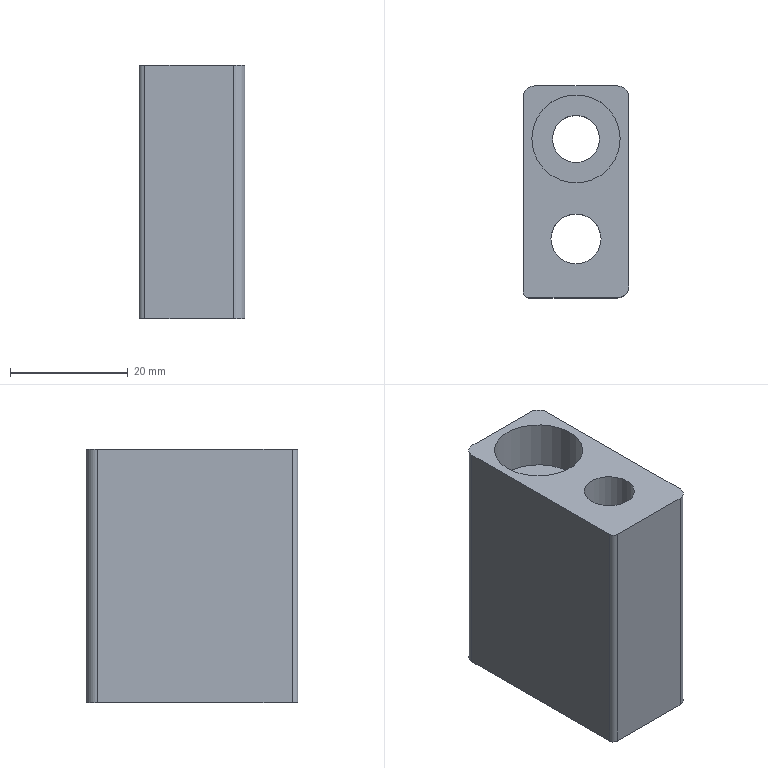Part | NX | features PH-18 2 | 1 solid | 16 faces | box 18 x 36 x 43 mm | volume 20467 mm3 | cylinder 8 | plane 8 | commonest cylinder face diameters 4 x3 2 x1 8.001 x1 8.5 x1 14.5 x1 15 x1
STEP:
#1=CARTESIAN_POINT('',(4143.236,-904.122,902.716));
#2=VERTEX_POINT('',#1);
#3=CARTESIAN_POINT('',(4145.236,-902.122,902.716));
#4=VERTEX_POINT('',#3);
#5=CARTESIAN_POINT('',(4143.236,-902.122,902.716));
#6=DIRECTION('',(0.,0.,-1.));
#7=DIRECTION('',(-1.,0.,0.));
#8=AXIS2_PLACEMENT_3D('',#5,#6,#7);
#9=CIRCLE('',#8,2.);
#10=EDGE_CURVE('',#2,#4,#9,.F.);
#11=ORIENTED_EDGE('',*,*,#10,.T.);
#12=CARTESIAN_POINT('',(4145.236,-902.122,945.716));
#13=VERTEX_POINT('',#12);
#14=CARTESIAN_POINT('',(4145.236,-902.122,915.716));
#15=DIRECTION('',(0.,0.,1.));
#16=VECTOR('',#15,1000.);
#17=LINE('',#14,#16);
#18=EDGE_CURVE('',#4,#13,#17,.T.);
#19=ORIENTED_EDGE('',*,*,#18,.T.);
#20=CARTESIAN_POINT('',(4143.236,-904.122,945.716));
#21=VERTEX_POINT('',#20);
#22=CARTESIAN_POINT('',(4143.236,-902.122,945.716));
#23=DIRECTION('',(0.,0.,-1.));
#24=DIRECTION('',(1.,0.,0.));
#25=AXIS2_PLACEMENT_3D('',#22,#23,#24);
#26=CIRCLE('',#25,2.);
#27=EDGE_CURVE('',#13,#21,#26,.T.);
#28=ORIENTED_EDGE('',*,*,#27,.T.);
#29=CARTESIAN_POINT('',(4143.236,-904.122,915.716));
#30=DIRECTION('',(0.,0.,1.));
#31=VECTOR('',#30,1000.);
#32=LINE('',#29,#31);
#33=EDGE_CURVE('',#21,#2,#32,.F.);
#34=ORIENTED_EDGE('',*,*,#33,.T.);
#35=EDGE_LOOP('',(#11,#19,#28,#34));
#36=FACE_BOUND('',#35,.T.);
#37=CARTESIAN_POINT('',(4143.236,-902.122,915.716));
#38=DIRECTION('',(0.,0.,1.));
#39=DIRECTION('',(1.,0.,0.));
#40=AXIS2_PLACEMENT_3D('',#37,#38,#39);
#41=CYLINDRICAL_SURFACE('',#40,2.);
#42=ADVANCED_FACE('',(#36),#41,.T.);
#43=CARTESIAN_POINT('',(4143.236,-868.122,902.716));
#44=VERTEX_POINT('',#43);
#45=CARTESIAN_POINT('',(4129.236,-868.122,902.716));
#46=VERTEX_POINT('',#45);
#47=CARTESIAN_POINT('',(4136.236,-868.122,902.716));
#48=DIRECTION('',(1.,0.,0.));
#49=VECTOR('',#48,1000.);
#50=LINE('',#47,#49);
#51=EDGE_CURVE('',#44,#46,#50,.F.);
#52=ORIENTED_EDGE('',*,*,#51,.T.);
#53=CARTESIAN_POINT('',(4129.236,-868.122,945.716));
#54=VERTEX_POINT('',#53);
#55=CARTESIAN_POINT('',(4129.236,-868.122,915.716));
#56=DIRECTION('',(0.,0.,1.));
#57=VECTOR('',#56,1000.);
#58=LINE('',#55,#57);
#59=EDGE_CURVE('',#54,#46,#58,.F.);
#60=ORIENTED_EDGE('',*,*,#59,.F.);
#61=CARTESIAN_POINT('',(4143.236,-868.122,945.716));
#62=VERTEX_POINT('',#61);
#63=CARTESIAN_POINT('',(4136.236,-868.122,945.716));
#64=DIRECTION('',(-1.,0.,0.));
#65=VECTOR('',#64,1000.);
#66=LINE('',#63,#65);
#67=EDGE_CURVE('',#54,#62,#66,.F.);
#68=ORIENTED_EDGE('',*,*,#67,.T.);
#69=CARTESIAN_POINT('',(4143.236,-868.122,915.716));
#70=DIRECTION('',(0.,0.,1.));
#71=VECTOR('',#70,1000.);
#72=LINE('',#69,#71);
#73=EDGE_CURVE('',#44,#62,#72,.T.);
#74=ORIENTED_EDGE('',*,*,#73,.F.);
#75=EDGE_LOOP('',(#52,#60,#68,#74));
#76=FACE_BOUND('',#75,.T.);
#77=CARTESIAN_POINT('',(4136.236,-868.122,915.716));
#78=DIRECTION('',(0.,1.,0.));
#79=DIRECTION('',(0.,0.,-1.));
#80=AXIS2_PLACEMENT_3D('',#77,#78,#79);
#81=PLANE('',#80);
#82=ADVANCED_FACE('',(#76),#81,.T.);
#83=CARTESIAN_POINT('',(4127.236,-870.122,902.716));
#84=VERTEX_POINT('',#83);
#85=CARTESIAN_POINT('',(4129.236,-870.122,902.716));
#86=DIRECTION('',(0.,0.,-1.));
#87=DIRECTION('',(-1.,0.,0.));
#88=AXIS2_PLACEMENT_3D('',#85,#86,#87);
#89=CIRCLE('',#88,2.);
#90=EDGE_CURVE('',#46,#84,#89,.F.);
#91=ORIENTED_EDGE('',*,*,#90,.T.);
#92=CARTESIAN_POINT('',(4127.236,-870.122,945.716));
#93=VERTEX_POINT('',#92);
#94=CARTESIAN_POINT('',(4127.236,-870.122,915.716));
#95=DIRECTION('',(0.,0.,1.));
#96=VECTOR('',#95,1000.);
#97=LINE('',#94,#96);
#98=EDGE_CURVE('',#84,#93,#97,.T.);
#99=ORIENTED_EDGE('',*,*,#98,.T.);
#100=CARTESIAN_POINT('',(4129.236,-870.122,945.716));
#101=DIRECTION('',(0.,0.,-1.));
#102=DIRECTION('',(1.,0.,0.));
#103=AXIS2_PLACEMENT_3D('',#100,#101,#102);
#104=CIRCLE('',#103,2.);
#105=EDGE_CURVE('',#93,#54,#104,.T.);
#106=ORIENTED_EDGE('',*,*,#105,.T.);
#107=ORIENTED_EDGE('',*,*,#59,.T.);
#108=EDGE_LOOP('',(#91,#99,#106,#107));
#109=FACE_BOUND('',#108,.T.);
#110=CARTESIAN_POINT('',(4129.236,-870.122,915.716));
#111=DIRECTION('',(0.,0.,1.));
#112=DIRECTION('',(1.,0.,0.));
#113=AXIS2_PLACEMENT_3D('',#110,#111,#112);
#114=CYLINDRICAL_SURFACE('',#113,2.);
#115=ADVANCED_FACE('',(#109),#114,.T.);
#116=CARTESIAN_POINT('',(4127.236,-903.122,945.716));
#117=VERTEX_POINT('',#116);
#118=CARTESIAN_POINT('',(4127.236,-885.622,945.716));
#119=DIRECTION('',(0.,-1.,0.));
#120=VECTOR('',#119,1000.);
#121=LINE('',#118,#120);
#122=EDGE_CURVE('',#117,#93,#121,.F.);
#123=ORIENTED_EDGE('',*,*,#122,.T.);
#124=ORIENTED_EDGE('',*,*,#98,.F.);
#125=CARTESIAN_POINT('',(4127.236,-903.122,902.716));
#126=VERTEX_POINT('',#125);
#127=CARTESIAN_POINT('',(4127.236,-885.622,902.716));
#128=DIRECTION('',(0.,1.,0.));
#129=VECTOR('',#128,1000.);
#130=LINE('',#127,#129);
#131=EDGE_CURVE('',#126,#84,#130,.T.);
#132=ORIENTED_EDGE('',*,*,#131,.F.);
#133=CARTESIAN_POINT('',(4127.236,-903.122,915.716));
#134=DIRECTION('',(0.,0.,1.));
#135=VECTOR('',#134,1000.);
#136=LINE('',#133,#135);
#137=EDGE_CURVE('',#117,#126,#136,.F.);
#138=ORIENTED_EDGE('',*,*,#137,.F.);
#139=EDGE_LOOP('',(#123,#124,#132,#138));
#140=FACE_BOUND('',#139,.T.);
#141=CARTESIAN_POINT('',(4127.236,-885.622,915.716));
#142=DIRECTION('',(-1.,0.,0.));
#143=DIRECTION('',(0.,0.,1.));
#144=AXIS2_PLACEMENT_3D('',#141,#142,#143);
#145=PLANE('',#144);
#146=ADVANCED_FACE('',(#140),#145,.T.);
#147=CARTESIAN_POINT('',(4145.236,-870.122,902.716));
#148=VERTEX_POINT('',#147);
#149=CARTESIAN_POINT('',(4143.236,-870.122,902.716));
#150=DIRECTION('',(0.,0.,-1.));
#151=DIRECTION('',(-1.,0.,0.));
#152=AXIS2_PLACEMENT_3D('',#149,#150,#151);
#153=CIRCLE('',#152,2.);
#154=EDGE_CURVE('',#148,#44,#153,.F.);
#155=ORIENTED_EDGE('',*,*,#154,.T.);
#156=ORIENTED_EDGE('',*,*,#73,.T.);
#157=CARTESIAN_POINT('',(4145.236,-870.122,945.716));
#158=VERTEX_POINT('',#157);
#159=CARTESIAN_POINT('',(4143.236,-870.122,945.716));
#160=DIRECTION('',(0.,0.,-1.));
#161=DIRECTION('',(1.,0.,0.));
#162=AXIS2_PLACEMENT_3D('',#159,#160,#161);
#163=CIRCLE('',#162,2.);
#164=EDGE_CURVE('',#158,#62,#163,.F.);
#165=ORIENTED_EDGE('',*,*,#164,.F.);
#166=CARTESIAN_POINT('',(4145.236,-870.122,915.716));
#167=DIRECTION('',(0.,0.,1.));
#168=VECTOR('',#167,1000.);
#169=LINE('',#166,#168);
#170=EDGE_CURVE('',#158,#148,#169,.F.);
#171=ORIENTED_EDGE('',*,*,#170,.T.);
#172=EDGE_LOOP('',(#155,#156,#165,#171));
#173=FACE_BOUND('',#172,.T.);
#174=CARTESIAN_POINT('',(4143.236,-870.122,915.716));
#175=DIRECTION('',(0.,0.,1.));
#176=DIRECTION('',(1.,0.,0.));
#177=AXIS2_PLACEMENT_3D('',#174,#175,#176);
#178=CYLINDRICAL_SURFACE('',#177,2.);
#179=ADVANCED_FACE('',(#173),#178,.T.);
#180=CARTESIAN_POINT('',(4128.236,-904.122,902.716));
#181=VERTEX_POINT('',#180);
#182=CARTESIAN_POINT('',(4136.236,-904.122,902.716));
#183=DIRECTION('',(-1.,0.,0.));
#184=VECTOR('',#183,1000.);
#185=LINE('',#182,#184);
#186=EDGE_CURVE('',#181,#2,#185,.F.);
#187=ORIENTED_EDGE('',*,*,#186,.T.);
#188=ORIENTED_EDGE('',*,*,#33,.F.);
#189=CARTESIAN_POINT('',(4128.236,-904.122,945.716));
#190=VERTEX_POINT('',#189);
#191=CARTESIAN_POINT('',(4136.236,-904.122,945.716));
#192=DIRECTION('',(1.,0.,0.));
#193=VECTOR('',#192,1000.);
#194=LINE('',#191,#193);
#195=EDGE_CURVE('',#21,#190,#194,.F.);
#196=ORIENTED_EDGE('',*,*,#195,.T.);
#197=CARTESIAN_POINT('',(4128.236,-904.122,915.716));
#198=DIRECTION('',(0.,0.,1.));
#199=VECTOR('',#198,1000.);
#200=LINE('',#197,#199);
#201=EDGE_CURVE('',#181,#190,#200,.T.);
#202=ORIENTED_EDGE('',*,*,#201,.F.);
#203=EDGE_LOOP('',(#187,#188,#196,#202));
#204=FACE_BOUND('',#203,.T.);
#205=CARTESIAN_POINT('',(4136.236,-904.122,915.716));
#206=DIRECTION('',(0.,-1.,0.));
#207=DIRECTION('',(0.,0.,1.));
#208=AXIS2_PLACEMENT_3D('',#205,#206,#207);
#209=PLANE('',#208);
#210=ADVANCED_FACE('',(#204),#209,.T.);
#211=CARTESIAN_POINT('',(4145.236,-885.622,902.716));
#212=DIRECTION('',(0.,-1.,0.));
#213=VECTOR('',#212,1000.);
#214=LINE('',#211,#213);
#215=EDGE_CURVE('',#4,#148,#214,.F.);
#216=ORIENTED_EDGE('',*,*,#215,.T.);
#217=ORIENTED_EDGE('',*,*,#170,.F.);
#218=CARTESIAN_POINT('',(4145.236,-885.622,945.716));
#219=DIRECTION('',(0.,1.,0.));
#220=VECTOR('',#219,1000.);
#221=LINE('',#218,#220);
#222=EDGE_CURVE('',#158,#13,#221,.F.);
#223=ORIENTED_EDGE('',*,*,#222,.T.);
#224=ORIENTED_EDGE('',*,*,#18,.F.);
#225=EDGE_LOOP('',(#216,#217,#223,#224));
#226=FACE_BOUND('',#225,.T.);
#227=CARTESIAN_POINT('',(4145.236,-885.622,915.716));
#228=DIRECTION('',(1.,0.,0.));
#229=DIRECTION('',(0.,0.,-1.));
#230=AXIS2_PLACEMENT_3D('',#227,#228,#229);
#231=PLANE('',#230);
#232=ADVANCED_FACE('',(#226),#231,.T.);
#233=CARTESIAN_POINT('',(4128.236,-903.122,902.716));
#234=DIRECTION('',(0.,0.,-1.));
#235=DIRECTION('',(-1.,0.,0.));
#236=AXIS2_PLACEMENT_3D('',#233,#234,#235);
#237=CIRCLE('',#236,1.);
#238=EDGE_CURVE('',#126,#181,#237,.F.);
#239=ORIENTED_EDGE('',*,*,#238,.T.);
#240=ORIENTED_EDGE('',*,*,#201,.T.);
#241=CARTESIAN_POINT('',(4128.236,-903.122,945.716));
#242=DIRECTION('',(0.,0.,-1.));
#243=DIRECTION('',(1.,0.,0.));
#244=AXIS2_PLACEMENT_3D('',#241,#242,#243);
#245=CIRCLE('',#244,1.);
#246=EDGE_CURVE('',#190,#117,#245,.T.);
#247=ORIENTED_EDGE('',*,*,#246,.T.);
#248=ORIENTED_EDGE('',*,*,#137,.T.);
#249=EDGE_LOOP('',(#239,#240,#247,#248));
#250=FACE_BOUND('',#249,.T.);
#251=CARTESIAN_POINT('',(4128.236,-903.122,915.716));
#252=DIRECTION('',(0.,0.,1.));
#253=DIRECTION('',(1.,0.,0.));
#254=AXIS2_PLACEMENT_3D('',#251,#252,#253);
#255=CYLINDRICAL_SURFACE('',#254,1.);
#256=ADVANCED_FACE('',(#250),#255,.T.);
#257=CARTESIAN_POINT('',(4132.236,-877.122,902.716));
#258=VERTEX_POINT('',#257);
#259=CARTESIAN_POINT('',(4136.236,-877.122,902.716));
#260=DIRECTION('',(0.,0.,-1.));
#261=DIRECTION('',(-1.,0.,0.));
#262=AXIS2_PLACEMENT_3D('',#259,#260,#261);
#263=CIRCLE('',#262,4.);
#264=EDGE_CURVE('',#258,#258,#263,.T.);
#265=ORIENTED_EDGE('',*,*,#264,.T.);
#266=EDGE_LOOP('',(#265));
#267=FACE_BOUND('',#266,.T.);
#268=CARTESIAN_POINT('',(4132.236,-877.122,937.416));
#269=VERTEX_POINT('',#268);
#270=CARTESIAN_POINT('',(4136.236,-877.122,937.416));
#271=DIRECTION('',(0.,0.,-1.));
#272=DIRECTION('',(-1.,0.,0.));
#273=AXIS2_PLACEMENT_3D('',#270,#271,#272);
#274=CIRCLE('',#273,4.);
#275=EDGE_CURVE('',#269,#269,#274,.T.);
#276=ORIENTED_EDGE('',*,*,#275,.F.);
#277=EDGE_LOOP('',(#276));
#278=FACE_BOUND('',#277,.T.);
#279=CARTESIAN_POINT('',(4136.236,-877.122,945.716));
#280=DIRECTION('',(0.,0.,-1.));
#281=DIRECTION('',(1.,0.,0.));
#282=AXIS2_PLACEMENT_3D('',#279,#280,#281);
#283=CYLINDRICAL_SURFACE('',#282,4.);
#284=ADVANCED_FACE('',(#267,#278),#283,.F.);
#285=CARTESIAN_POINT('',(4143.486,-894.122,902.716));
#286=VERTEX_POINT('',#285);
#287=CARTESIAN_POINT('',(4136.236,-894.122,902.716));
#288=DIRECTION('',(0.,0.,1.));
#289=DIRECTION('',(1.,0.,0.));
#290=AXIS2_PLACEMENT_3D('',#287,#288,#289);
#291=CIRCLE('',#290,7.25);
#292=EDGE_CURVE('',#286,#286,#291,.T.);
#293=ORIENTED_EDGE('',*,*,#292,.T.);
#294=EDGE_LOOP('',(#293));
#295=FACE_BOUND('',#294,.T.);
#296=ORIENTED_EDGE('',*,*,#154,.F.);
#297=ORIENTED_EDGE('',*,*,#215,.F.);
#298=ORIENTED_EDGE('',*,*,#10,.F.);
#299=ORIENTED_EDGE('',*,*,#186,.F.);
#300=ORIENTED_EDGE('',*,*,#238,.F.);
#301=ORIENTED_EDGE('',*,*,#131,.T.);
#302=ORIENTED_EDGE('',*,*,#90,.F.);
#303=ORIENTED_EDGE('',*,*,#51,.F.);
#304=EDGE_LOOP('',(#296,#297,#298,#299,#300,#301,#302,#303));
#305=FACE_BOUND('',#304,.T.);
#306=ORIENTED_EDGE('',*,*,#264,.F.);
#307=EDGE_LOOP('',(#306));
#308=FACE_BOUND('',#307,.T.);
#309=CARTESIAN_POINT('',(4123.486,-858.122,902.716));
#310=DIRECTION('',(0.,0.,-1.));
#311=DIRECTION('',(-1.,0.,0.));
#312=AXIS2_PLACEMENT_3D('',#309,#310,#311);
#313=PLANE('',#312);
#314=ADVANCED_FACE('',(#295,#305,#308),#313,.T.);
#315=ORIENTED_EDGE('',*,*,#275,.T.);
#316=EDGE_LOOP('',(#315));
#317=FACE_BOUND('',#316,.T.);
#318=CARTESIAN_POINT('',(4143.736,-877.122,937.416));
#319=VERTEX_POINT('',#318);
#320=CARTESIAN_POINT('',(4136.236,-877.122,937.416));
#321=DIRECTION('',(0.,0.,1.));
#322=DIRECTION('',(1.,0.,0.));
#323=AXIS2_PLACEMENT_3D('',#320,#321,#322);
#324=CIRCLE('',#323,7.5);
#325=EDGE_CURVE('',#319,#319,#324,.T.);
#326=ORIENTED_EDGE('',*,*,#325,.T.);
#327=EDGE_LOOP('',(#326));
#328=FACE_BOUND('',#327,.T.);
#329=CARTESIAN_POINT('',(4136.236,-877.122,937.416));
#330=DIRECTION('',(0.,0.,-1.));
#331=DIRECTION('',(-1.,0.,0.));
#332=AXIS2_PLACEMENT_3D('',#329,#330,#331);
#333=PLANE('',#332);
#334=ADVANCED_FACE('',(#317,#328),#333,.F.);
#335=CARTESIAN_POINT('',(4143.736,-877.122,945.716));
#336=VERTEX_POINT('',#335);
#337=CARTESIAN_POINT('',(4136.236,-877.122,945.716));
#338=DIRECTION('',(0.,0.,-1.));
#339=DIRECTION('',(1.,0.,0.));
#340=AXIS2_PLACEMENT_3D('',#337,#338,#339);
#341=CIRCLE('',#340,7.5);
#342=EDGE_CURVE('',#336,#336,#341,.T.);
#343=ORIENTED_EDGE('',*,*,#342,.F.);
#344=EDGE_LOOP('',(#343));
#345=FACE_BOUND('',#344,.T.);
#346=ORIENTED_EDGE('',*,*,#325,.F.);
#347=EDGE_LOOP('',(#346));
#348=FACE_BOUND('',#347,.T.);
#349=CARTESIAN_POINT('',(4136.236,-877.122,945.716));
#350=DIRECTION('',(0.,0.,-1.));
#351=DIRECTION('',(1.,0.,0.));
#352=AXIS2_PLACEMENT_3D('',#349,#350,#351);
#353=CYLINDRICAL_SURFACE('',#352,7.5);
#354=ADVANCED_FACE('',(#345,#348),#353,.F.);
#355=CARTESIAN_POINT('',(4140.486,-894.122,945.716));
#356=VERTEX_POINT('',#355);
#357=CARTESIAN_POINT('',(4136.236,-894.122,945.716));
#358=DIRECTION('',(0.,0.,1.));
#359=DIRECTION('',(1.,0.,0.));
#360=AXIS2_PLACEMENT_3D('',#357,#358,#359);
#361=CIRCLE('',#360,4.25);
#362=EDGE_CURVE('',#356,#356,#361,.T.);
#363=ORIENTED_EDGE('',*,*,#362,.F.);
#364=EDGE_LOOP('',(#363));
#365=FACE_BOUND('',#364,.T.);
#366=ORIENTED_EDGE('',*,*,#164,.T.);
#367=ORIENTED_EDGE('',*,*,#67,.F.);
#368=ORIENTED_EDGE('',*,*,#105,.F.);
#369=ORIENTED_EDGE('',*,*,#122,.F.);
#370=ORIENTED_EDGE('',*,*,#246,.F.);
#371=ORIENTED_EDGE('',*,*,#195,.F.);
#372=ORIENTED_EDGE('',*,*,#27,.F.);
#373=ORIENTED_EDGE('',*,*,#222,.F.);
#374=EDGE_LOOP('',(#366,#367,#368,#369,#370,#371,#372,#373));
#375=FACE_BOUND('',#374,.T.);
#376=ORIENTED_EDGE('',*,*,#342,.T.);
#377=EDGE_LOOP('',(#376));
#378=FACE_BOUND('',#377,.T.);
#379=CARTESIAN_POINT('',(4123.486,-858.122,945.716));
#380=DIRECTION('',(0.,0.,1.));
#381=DIRECTION('',(1.,0.,0.));
#382=AXIS2_PLACEMENT_3D('',#379,#380,#381);
#383=PLANE('',#382);
#384=ADVANCED_FACE('',(#365,#375,#378),#383,.T.);
#385=ORIENTED_EDGE('',*,*,#362,.T.);
#386=EDGE_LOOP('',(#385));
#387=FACE_BOUND('',#386,.T.);
#388=CARTESIAN_POINT('',(4140.486,-894.122,917.716));
#389=VERTEX_POINT('',#388);
#390=CARTESIAN_POINT('',(4136.236,-894.122,917.716));
#391=DIRECTION('',(0.,0.,1.));
#392=DIRECTION('',(1.,0.,0.));
#393=AXIS2_PLACEMENT_3D('',#390,#391,#392);
#394=CIRCLE('',#393,4.25);
#395=EDGE_CURVE('',#389,#389,#394,.T.);
#396=ORIENTED_EDGE('',*,*,#395,.F.);
#397=EDGE_LOOP('',(#396));
#398=FACE_BOUND('',#397,.T.);
#399=CARTESIAN_POINT('',(4136.236,-894.122,902.716));
#400=DIRECTION('',(0.,0.,1.));
#401=DIRECTION('',(1.,0.,0.));
#402=AXIS2_PLACEMENT_3D('',#399,#400,#401);
#403=CYLINDRICAL_SURFACE('',#402,4.25);
#404=ADVANCED_FACE('',(#387,#398),#403,.F.);
#405=ORIENTED_EDGE('',*,*,#395,.T.);
#406=EDGE_LOOP('',(#405));
#407=FACE_BOUND('',#406,.T.);
#408=CARTESIAN_POINT('',(4143.486,-894.122,917.716));
#409=VERTEX_POINT('',#408);
#410=CARTESIAN_POINT('',(4136.236,-894.122,917.716));
#411=DIRECTION('',(0.,0.,-1.));
#412=DIRECTION('',(1.,0.,0.));
#413=AXIS2_PLACEMENT_3D('',#410,#411,#412);
#414=CIRCLE('',#413,7.25);
#415=EDGE_CURVE('',#409,#409,#414,.F.);
#416=ORIENTED_EDGE('',*,*,#415,.F.);
#417=EDGE_LOOP('',(#416));
#418=FACE_BOUND('',#417,.T.);
#419=CARTESIAN_POINT('',(4136.236,-894.122,917.716));
#420=DIRECTION('',(0.,0.,1.));
#421=DIRECTION('',(1.,0.,0.));
#422=AXIS2_PLACEMENT_3D('',#419,#420,#421);
#423=PLANE('',#422);
#424=ADVANCED_FACE('',(#407,#418),#423,.F.);
#425=ORIENTED_EDGE('',*,*,#415,.T.);
#426=EDGE_LOOP('',(#425));
#427=FACE_BOUND('',#426,.T.);
#428=ORIENTED_EDGE('',*,*,#292,.F.);
#429=EDGE_LOOP('',(#428));
#430=FACE_BOUND('',#429,.T.);
#431=CARTESIAN_POINT('',(4136.236,-894.122,902.716));
#432=DIRECTION('',(0.,0.,1.));
#433=DIRECTION('',(1.,0.,0.));
#434=AXIS2_PLACEMENT_3D('',#431,#432,#433);
#435=CYLINDRICAL_SURFACE('',#434,7.25);
#436=ADVANCED_FACE('',(#427,#430),#435,.F.);
#437=CLOSED_SHELL('',(#42,#82,#115,#146,#179,#210,#232,#256,#284,#314,#334,#354,#384,#404,#424,#436));
#438=MANIFOLD_SOLID_BREP('',#437);
#439=(LENGTH_UNIT()NAMED_UNIT(*)SI_UNIT(.MILLI.,.METRE.));
#440=UNCERTAINTY_MEASURE_WITH_UNIT(LENGTH_MEASURE(0.00001),#439,'','');
#441=(NAMED_UNIT(*)PLANE_ANGLE_UNIT()SI_UNIT($,.RADIAN.));
#442=(NAMED_UNIT(*)SI_UNIT($,.STERADIAN.)SOLID_ANGLE_UNIT());
#443=(GEOMETRIC_REPRESENTATION_CONTEXT(3)GLOBAL_UNCERTAINTY_ASSIGNED_CONTEXT((#440))GLOBAL_UNIT_ASSIGNED_CONTEXT((#439,#441,#442))REPRESENTATION_CONTEXT('',''));
#444=ADVANCED_BREP_SHAPE_REPRESENTATION('',(#438),#443);